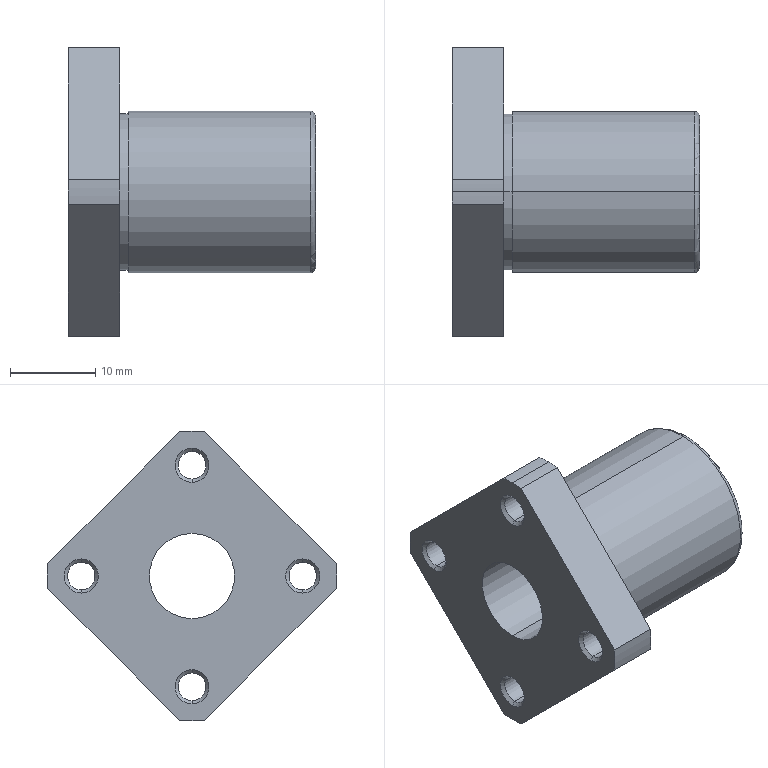Part | STEP file | LHTS10_default | 1 solid | 45 faces | box 29 x 34 x 34 mm | volume 8025 mm3 | cylinder 19 | cone 16 | plane 8 | torus 2 | commonest cylinder face diameters 3.242 x8 34 x5 10 x2 18.4 x2 19 x2